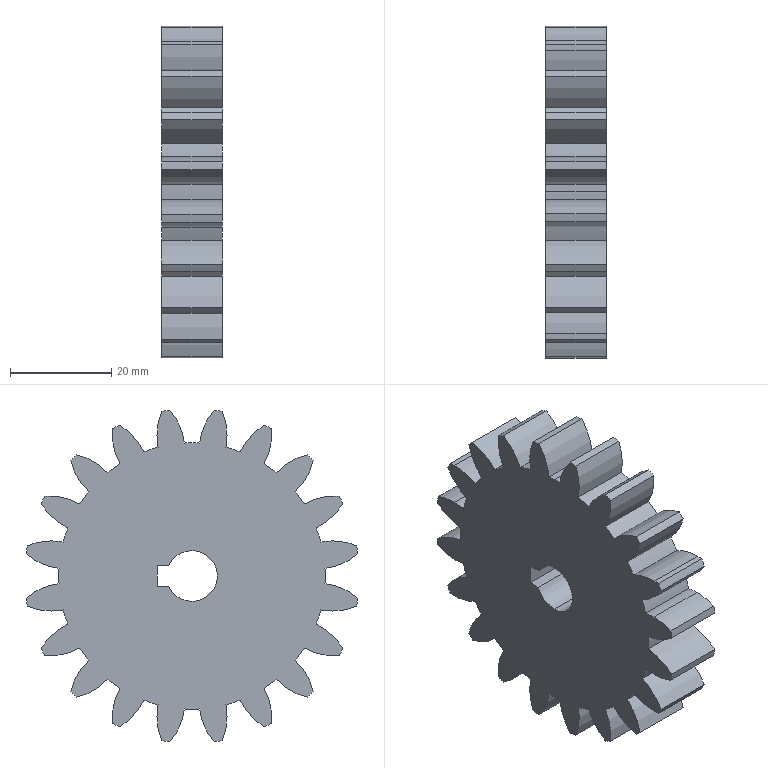Part | SolidWorks | features BaseBody 1 | 1 solid | 93 faces | box 12 x 65.416 x 65.416 mm | volume 31703 mm3 | cylinder 88 | plane 5 | commonest cylinder face diameters 24 x44 52.498 x21 66 x20 10 x3